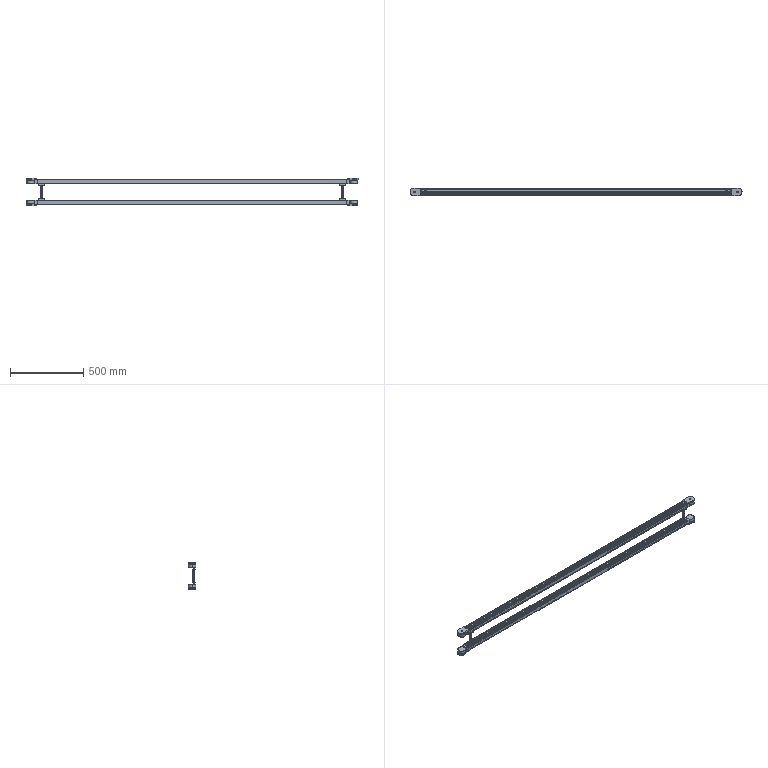Part | STEP file | Guide wheel mechanism revised.sldasm-Part-72 | 1 solid | 921 faces | box 2260 x 54 x 186 mm | volume 4417839 mm3 | plane 703 | cylinder 194 | cone 24 | commonest cylinder face diameters 12.2 x32 54 x22 6 x16 6.4 x16 7.2 x16 10 x16